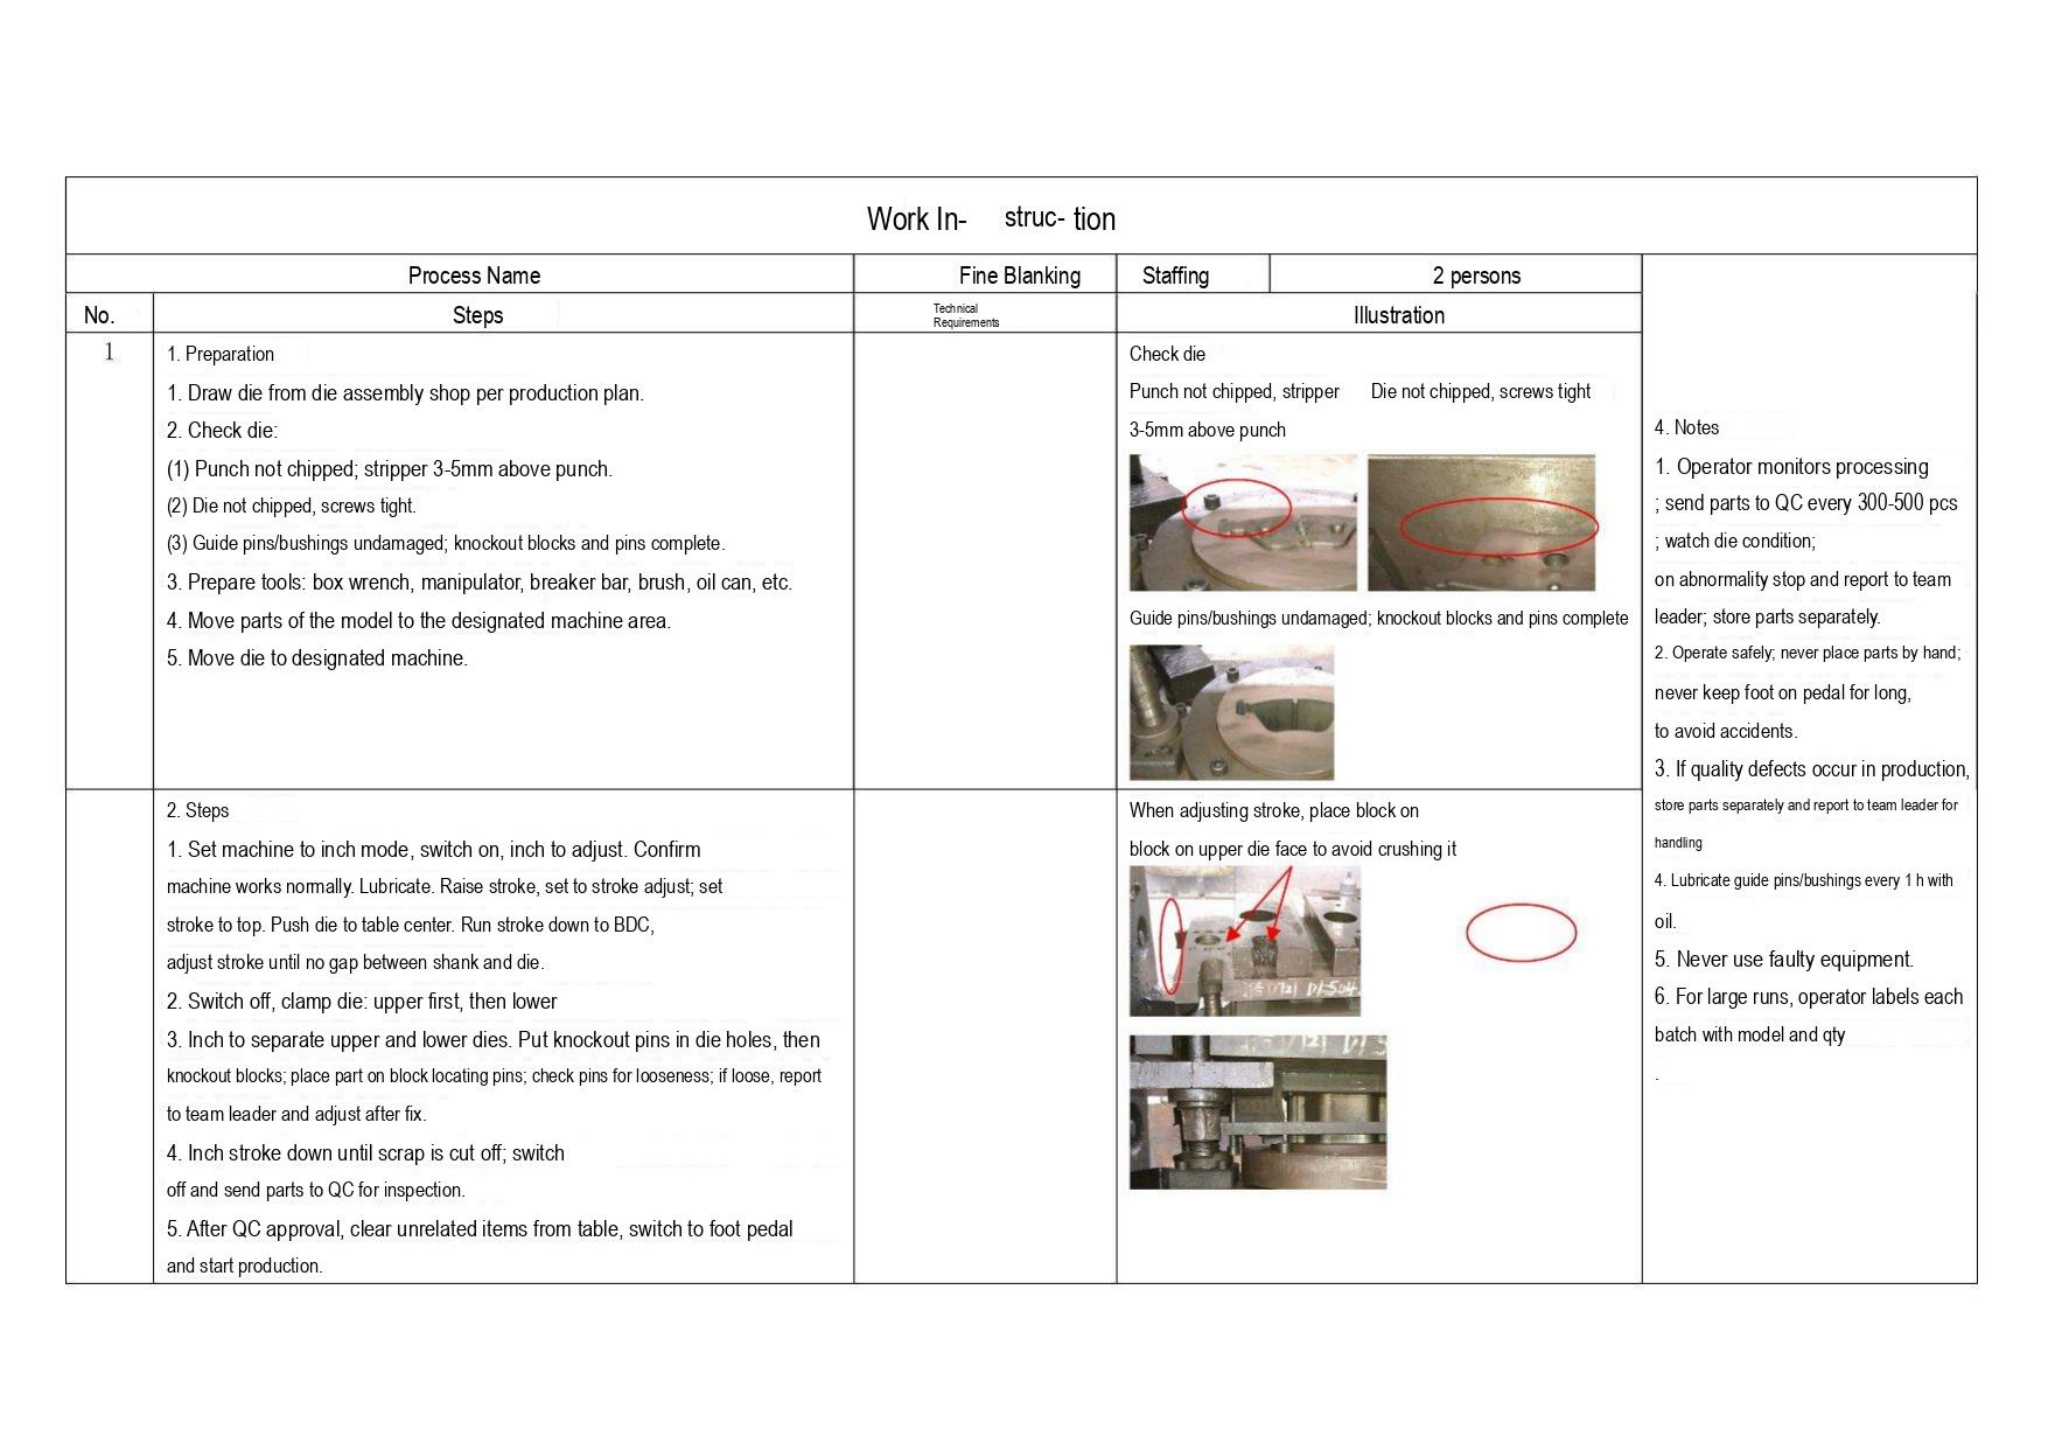# Work In- struc- tion

| Process Name | | Fine Blanking | Staffing | 2 persons |
|---|---|---|---|---|
| No. | Steps | Technical Requirements | Illustration | |
| 1 | 1. Preparation<br>1. Draw die from die assembly shop per production plan.<br>2. Check die:<br>(1) Punch not chipped; stripper 3-5mm above punch.<br>(2) Die not chipped, screws tight.<br>(3) Guide pins/bushings undamaged; knockout blocks and pins complete.<br>3. Prepare tools: box wrench, manipulator, breaker bar, brush, oil can, etc.<br>4. Move parts of the model to the designated machine area.<br>5. Move die to designated machine. | | Check die<br>Punch not chipped, stripper 3-5mm above punch<br>Die not chipped, screws tight<br>Guide pins/bushings undamaged; knockout blocks and pins complete | 4. Notes<br>1. Operator monitors processing<br>; send parts to QC every 300-500 pcs<br>; watch die condition;<br>on abnormality stop and report to team leader; store parts separately.<br>2. Operate safely; never place parts by hand;<br>never keep foot on pedal for long,<br>to avoid accidents.<br>3. If quality defects occur in production,<br>store parts separately and report to team leader for handling<br>4. Lubricate guide pins/bushings every 1 h with oil.<br>5. Never use faulty equipment.<br>6. For large runs, operator labels each batch with model and qty<br>. |
| | 2. Steps<br>1. Set machine to inch mode, switch on, inch to adjust. Confirm machine works normally. Lubricate. Raise stroke, set to stroke adjust; set stroke to top. Push die to table center. Run stroke down to BDC, adjust stroke until no gap between shank and die.<br>2. Switch off, clamp die: upper first, then lower<br>3. Inch to separate upper and lower dies. Put knockout pins in die holes, then knockout blocks; place part on block locating pins; check pins for looseness; if loose, report to team leader and adjust after fix.<br>4. Inch stroke down until scrap is cut off; switch off and send parts to QC for inspection.<br>5. After QC approval, clear unrelated items from table, switch to foot pedal and start production. | | When adjusting stroke, place block on block on upper die face to avoid crushing it | |
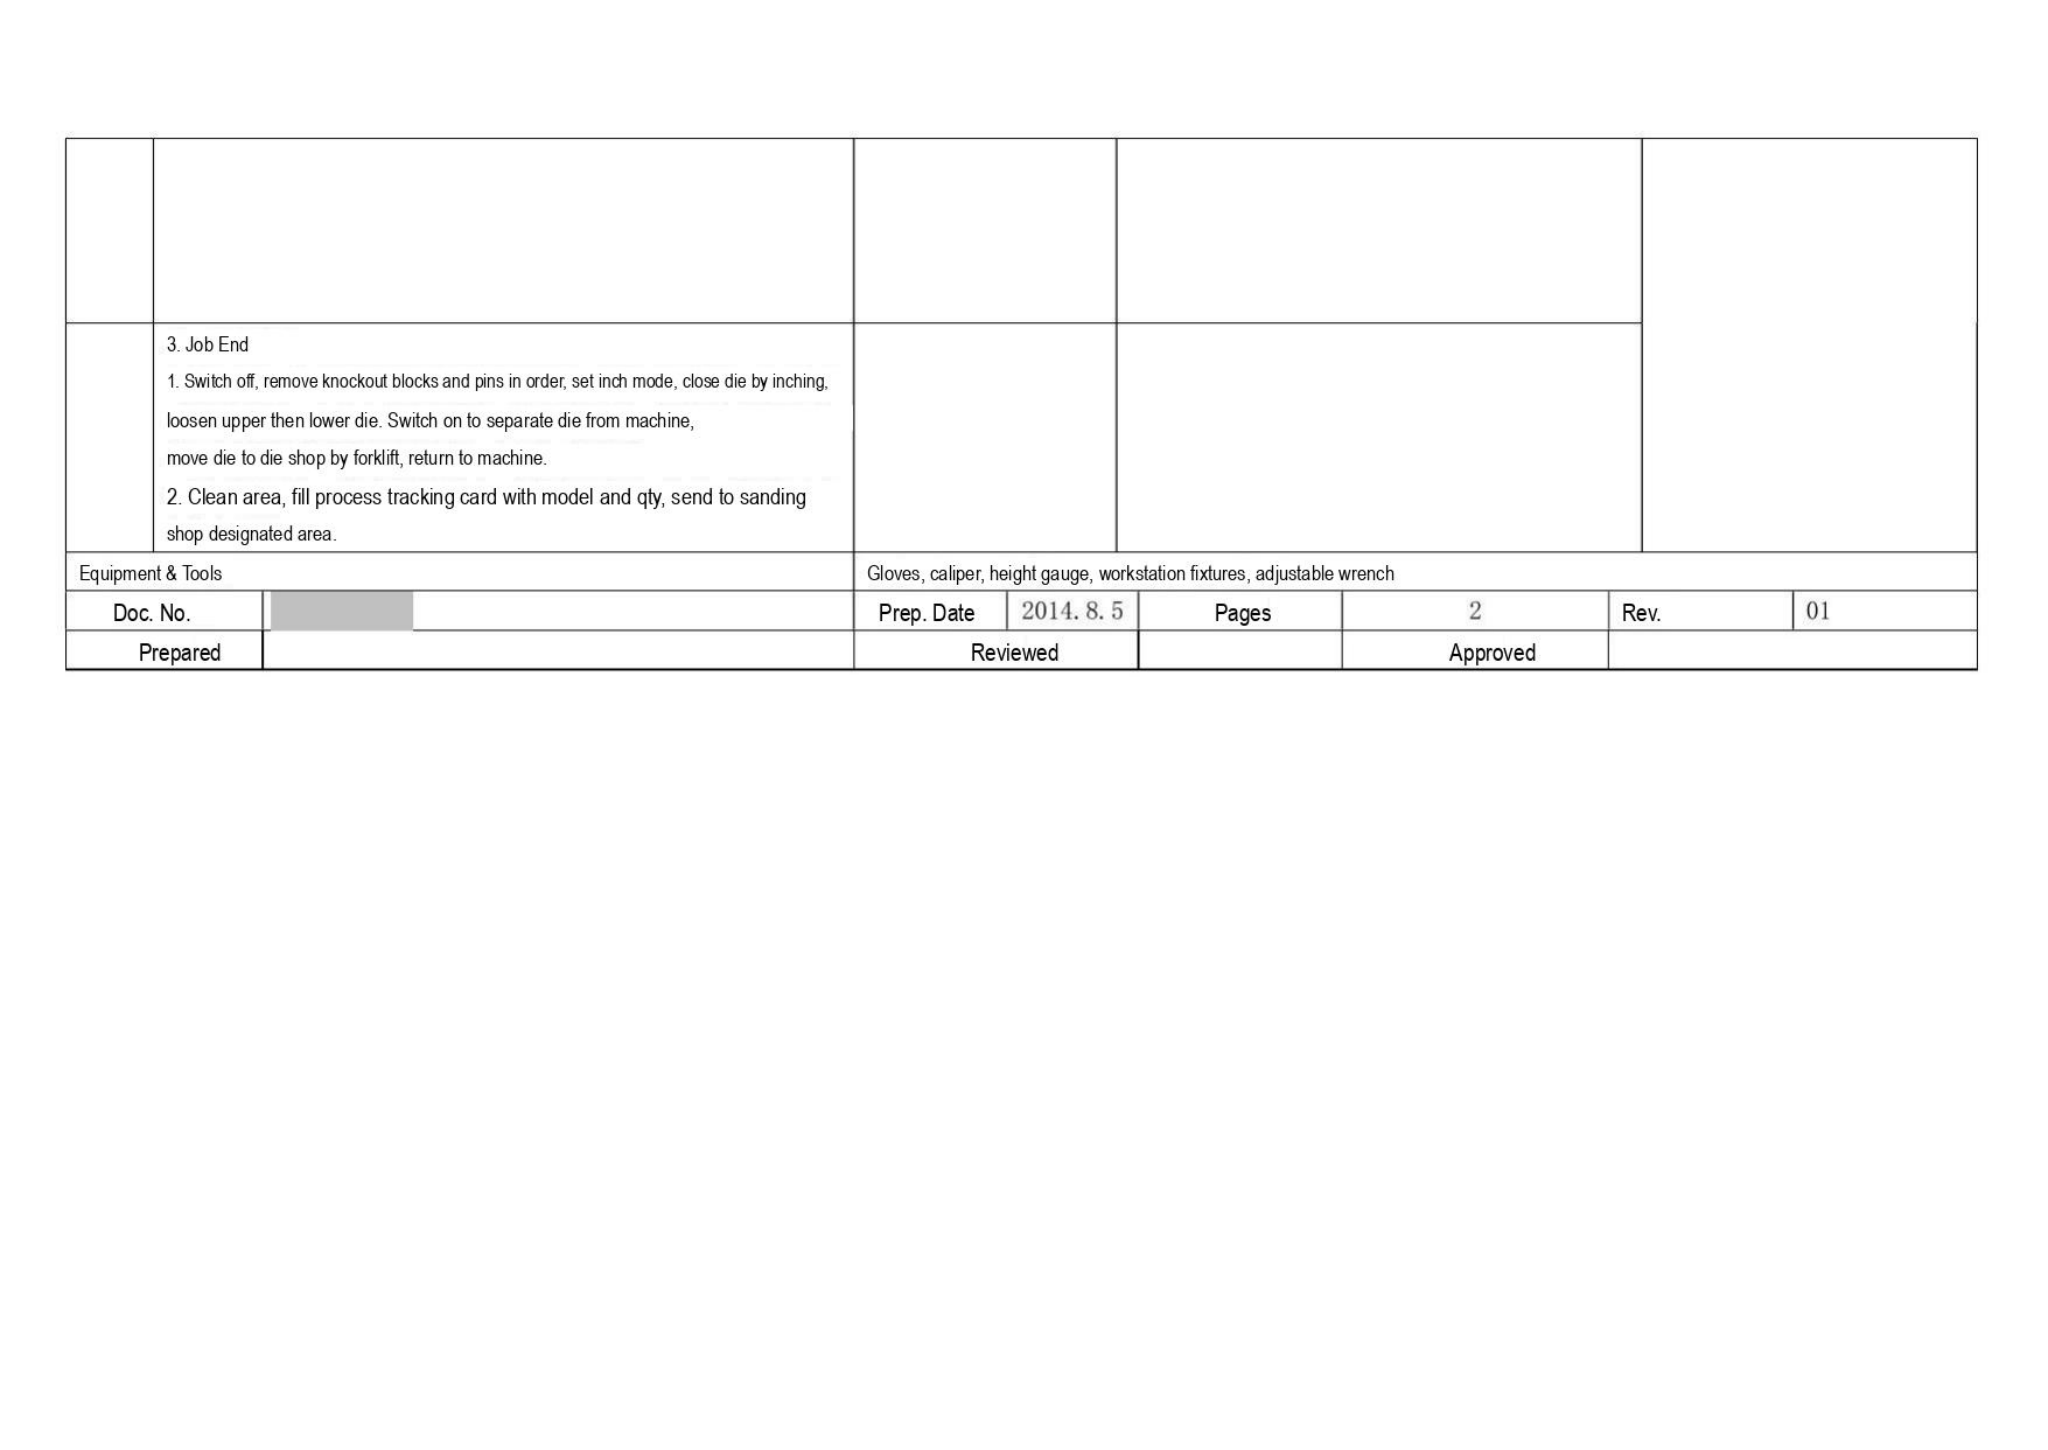| | | | | |
|---|---|---|---|---|
| | | | | |
| | 3. Job End<br>1. Switch off, remove knockout blocks and pins in order, set inch mode, close die by inching, loosen upper then lower die. Switch on to separate die from machine, move die to die shop by forklift, return to machine.<br>2. Clean area, fill process tracking card with model and qty, send to sanding shop designated area. | | | |

| | | | | | | | |
|---|---|---|---|---|---|---|---|
| Equipment & Tools | | Gloves, caliper, height gauge, workstation fixtures, adjustable wrench | | | | | |
| Doc. No. | | Prep. Date | 2014. 8. 5 | Pages | 2 | Rev. | 01 |
| Prepared | | Reviewed | | | Approved | | |